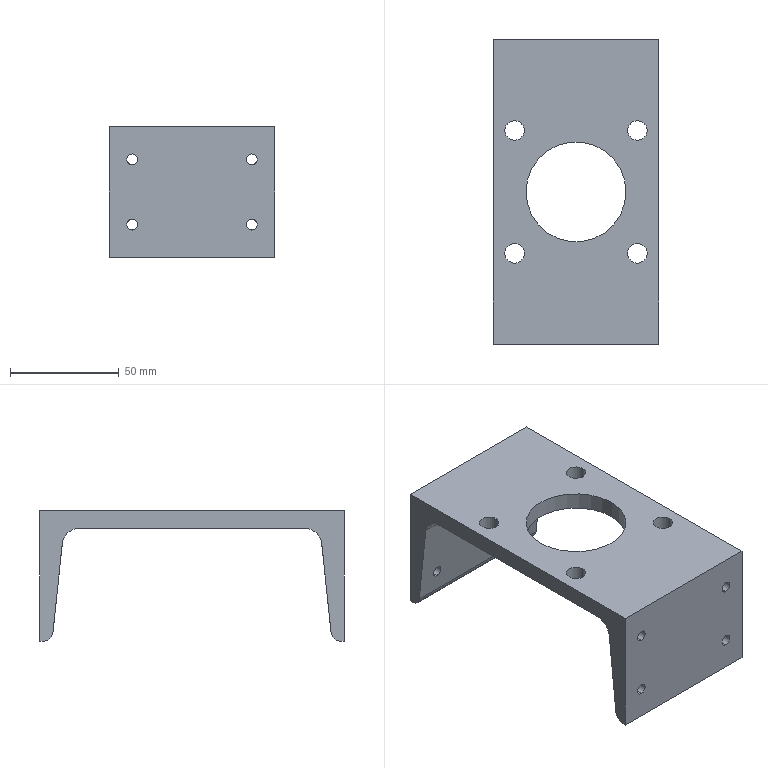Part | SolidWorks | features ICE 2, 3DProfileFeature 1, HoleWzd 1, WeldMemberFeat 1, WeldmentFeature 1 | 1 solid | 40 faces | box 76 x 140 x 60 mm | volume 135317 mm3 | cylinder 30 | plane 10 | commonest cylinder face diameters 5 x16 9 x10 16 x2 46 x2